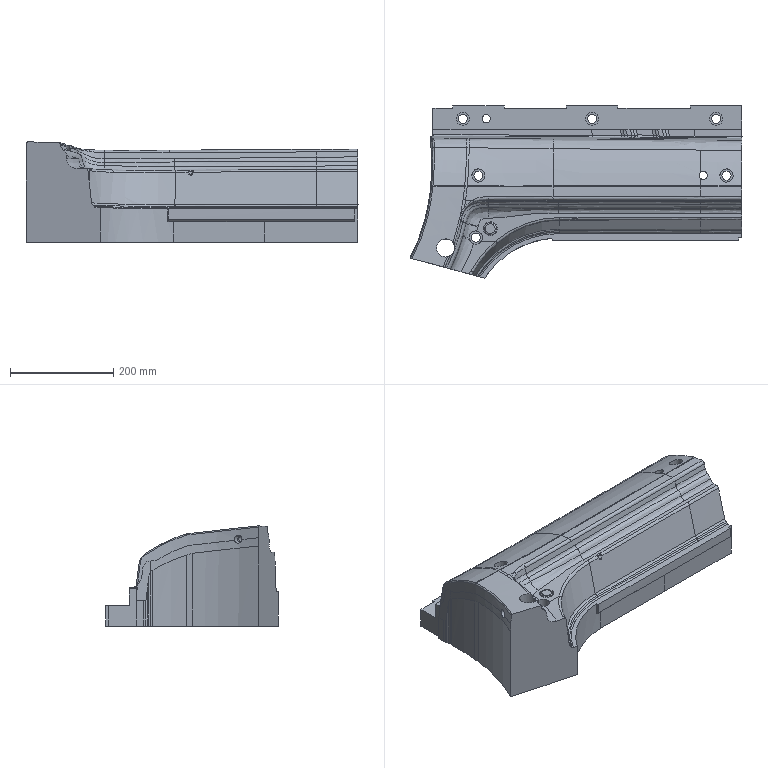Part | NX | features solid 2 | 1 solid | 220 faces | box 642.362 x 333.362 x 194.398 mm | volume 16208188 mm3 | spline 161 | plane 42 | cylinder 17 | commonest cylinder face diameters 17.5 x6 25.5 x6 16 x3 12 x1 35 x1